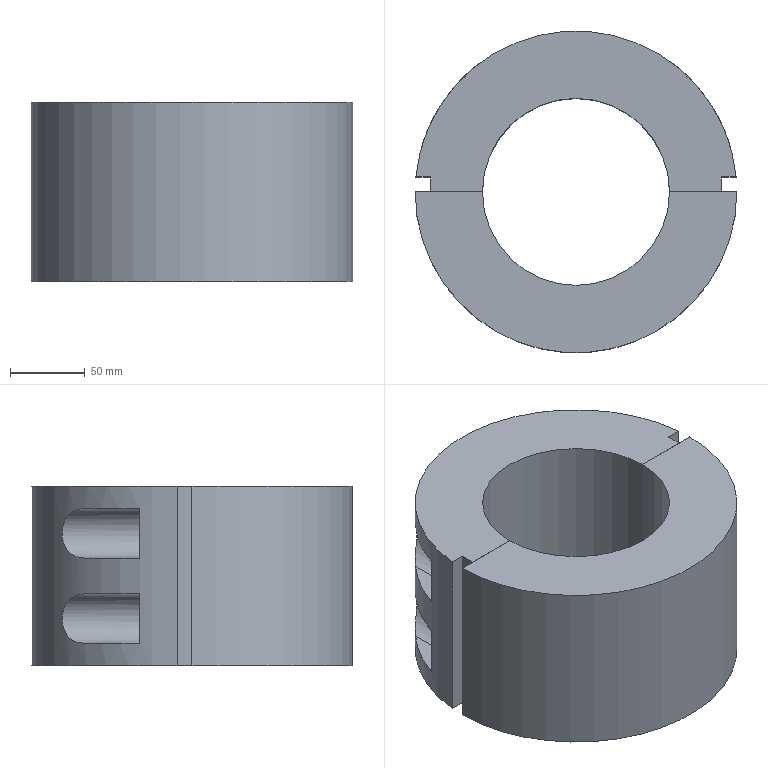NC program | NX | posted with a generic post | part box 215 x 215 x 120 mm
Lines 1 to 978 of 5839:
N10 G17 G21 G94 G90
(ZLEVEL_PROFILE , TOOL : D25)
N12 T01 M6
N14 G54
N16 G17 G0 G90 X-84.857 Y27.341 S1000 M3
N18 G43 Z30. H1
N20 Z-20.759
N22 G94 G1 X-80.33 Y25.016 F2000.
N24 G3 X-77.833 Y25.138 R2.5
N26 X-77.839 Y31.866 R4.
N28 X-80.336 Y31.984 R2.5
N30 G1 X-84.852 Y29.654
N32 G0 X-84.889 Y27.512 Z-21.109
N34 G1 X-80.453 Y25.029
N36 G3 X-77.954 Y25.063 R2.5
N38 X-77.949 Y31.934 R4.
N40 X-80.449 Y31.971 R2.5
N42 G1 X-84.894 Y29.491
N44 G0 X-84.922 Y27.671 Z-21.458
N46 G1 X-80.565 Y25.046
N48 G3 X-78.065 Y24.999 R2.5
N50 X-78.061 Y31.999 R4.
N52 X-80.561 Y31.955 R2.5
N54 G1 X-84.925 Y29.331
N56 G0 X-84.953 Y27.824 Z-21.808
N58 G1 X-80.668 Y25.064
N60 G3 X-78.171 Y24.943 R2.5
N62 X-78.173 Y32.058 R4.
N64 X-80.67 Y31.935 R2.5
N66 G1 X-84.947 Y29.176
N68 G0 X-84.96 Y27.979 Z-22.158
N70 G1 X-80.781 Y25.088
N72 G3 X-78.289 Y24.884 R2.5
N74 X-78.28 Y32.111 R4.
N76 X-80.773 Y31.914 R2.5
N78 G1 X-84.968 Y29.026
N80 G0 X-84.979 Y28.124 Z-22.507
N82 G1 X-80.876 Y25.111
N84 G3 X-78.391 Y24.838 R2.5
N86 X-78.397 Y32.165 R4.
N88 X-80.882 Y31.887 R2.5
N90 G1 X-84.975 Y28.872
N92 G0 X-84.991 Y28.266 Z-22.857
N94 G1 X-80.97 Y25.137
N96 G3 X-78.494 Y24.794 R2.5
N98 X-78.504 Y32.21 R4.
N100 X-80.979 Y31.86 R2.5
N102 G1 X-84.983 Y28.728
N104 G0 X-84.993 Y28.408 Z-23.206
N106 G1 X-81.068 Y25.167
N108 G3 X-78.603 Y24.752 R2.5
N110 X-78.601 Y32.247 R4.
N112 X-81.067 Y31.834 R2.5
N114 G1 X-84.994 Y28.592
N116 G0 X-89.054 Y32.079 Z-23.556
N118 G1 X-81.156 Y25.196
N120 G3 X-78.702 Y24.716 R2.5
N122 X-78.7 Y32.283 R4.
N124 X-81.154 Y31.804 R2.5
N126 G1 X-89.065 Y24.919
N128 G0 X-85.266 Y28.501 Z-23.906
N130 G1 X-81.25 Y25.231
N132 G3 X-78.811 Y24.681 R2.5
N134 X-78.811 Y32.319 R4.
N136 X-81.25 Y31.769 R2.5
N138 G1 X-85.266 Y28.501
N140 G0 X-85.496 Z-24.255
N142 G1 X-81.34 Y25.267
N144 G3 X-78.917 Y24.649 R2.5
N146 X-78.909 Y32.348 R4.
N148 X-81.333 Y31.736 R2.5
N150 G1 X-85.496 Y28.501
N152 G0 X-85.732 Y28.5 Z-24.605
N154 G1 X-81.42 Y25.301
N156 G3 X-79.014 Y24.623 R2.5
N158 X-79.008 Y32.375 R4.
N160 X-81.416 Y31.701 R2.5
N162 G1 X-85.732 Y28.5
N164 G0 X-85.978 Z-24.954
N166 G1 X-81.499 Y25.337
N168 G3 X-79.111 Y24.6 R2.5
N170 X-79.108 Y32.399 R4.
N172 X-81.497 Y31.664 R2.5
N174 G1 X-85.978 Y28.5
N176 G0 X-86.23 Z-25.304
N178 G1 X-81.574 Y25.374
N180 G3 X-79.203 Y24.58 R2.5
N182 X-79.208 Y32.421 R4.
N184 X-81.578 Y31.624 R2.5
N186 G1 X-86.23 Y28.5
N188 G0 X-86.491 Z-25.654
N190 G1 X-81.653 Y25.415
N192 G3 X-79.303 Y24.561 R2.5
N194 X-79.303 Y32.439 R4.
N196 X-81.653 Y31.585 R2.5
N198 G1 X-86.491 Y28.5
N200 G0 X-86.763 Z-26.003
N202 G1 X-81.714 Y25.448
N204 G3 X-79.381 Y24.548 R2.5
N206 X-79.385 Y32.452 R4.
N208 X-81.716 Y31.55 R2.5
N210 G1 X-86.763 Y28.5
N212 G0 X-87.061 Y28.501 Z-26.353
N214 G1 X-81.799 Y25.498
N216 G3 X-79.493 Y24.532 R2.5
N218 X-79.492 Y32.468 R4.
N220 X-81.798 Y31.503 R2.5
N222 G1 X-87.061 Y28.501
N224 G0 X-87.378 Y28.499 Z-26.702
N226 G1 X-81.868 Y25.54
N228 G3 X-79.585 Y24.522 R2.5
N230 X-79.67 Y32.486 R4.
N232 X-81.931 Y31.419 R2.5
N234 G1 X-87.378 Y28.499
N236 G0 X-87.666 Y28.5 Z-27.052
N238 G1 X-81.925 Y25.577
N240 G3 X-79.662 Y24.514 R2.5
N242 X-79.67 Y32.486 R4.
N244 X-81.931 Y31.419 R2.5
N246 G1 X-87.666 Y28.5
N248 G0 X-87.966 Z-27.402
N250 G1 X-81.991 Y25.621
N252 G3 X-79.752 Y24.508 R2.5
N254 X-79.769 Y32.493 R4.
N256 X-82.003 Y31.37 R2.5
N258 G1 X-87.966 Y28.5
N260 G0 X-88.287 Y28.501 Z-27.751
N262 G1 X-82.048 Y25.662
N264 G3 X-79.833 Y24.503 R2.5
N266 X-79.835 Y32.497 R4.
N268 X-82.05 Y31.337 R2.5
N270 G1 X-88.287 Y28.501
N272 G0 X-88.653 Z-28.101
N274 G1 X-82.114 Y25.71
N276 G3 X-79.926 Y24.501 R2.5
N278 X-79.927 Y32.499 R4.
N280 X-82.114 Y31.289 R2.5
N282 G1 X-88.653 Y28.501
N284 G0 X-89.027 Y28.5 Z-28.45
N286 G1 X-82.225 Y25.75
N288 G3 X-80.06 Y24.5 R2.5
N290 G1 X-80.
N292 G3 X-76. Y28.5 R4.
N294 X-80. Y32.5 R4.
N296 G1 X-80.112
N298 G3 X-82.277 Y31.25 R2.5
N300 G1 X-89.027 Y28.5
N302 G0 X-89.347 Y28.499 Z-28.8
N304 G1 X-82.598 Y25.75
N306 G3 X-80.433 Y24.5 R2.5
N308 G1 X-80.
N310 G3 X-76. Y28.5 R4.
N312 X-80. Y32.5 R4.
N314 G1 X-80.247
N316 G3 X-82.412 Y31.25 R2.5
N318 G1 X-89.347 Y28.499
N320 G0 X-89.666 Y28.5 Z-29.15
N322 G1 X-82.923 Y25.75
N324 G3 X-80.758 Y24.5 R2.5
N326 G1 X-80.
N328 G3 X-76. Y28.5 R4.
N330 X-80. Y32.5 R4.
N332 G1 X-80.654
N334 G3 X-82.819 Y31.25 R2.5
N336 G1 X-89.666 Y28.5
N338 G0 X-89.982 Y28.498 Z-29.499
N340 G1 X-83.238 Y25.75
N342 G3 X-81.073 Y24.5 R2.5
N344 G1 X-80.
N346 G3 X-76. Y28.5 R4.
N348 X-80. Y32.5 R4.
N350 G1 X-81.073
N352 G3 X-83.238 Y31.25 R2.5
N354 G1 X-89.982 Y28.498
N356 G0 X-90.302 Y28.502 Z-29.849
N358 G1 X-83.396 Y25.75
N360 G3 X-81.231 Y24.5 R2.5
N362 G1 X-80.
N364 G3 X-76. Y28.5 R4.
N366 X-80. Y32.5 R4.
N368 G1 X-81.24
N370 G3 X-83.405 Y31.25 R2.5
N372 G1 X-90.302 Y28.502
N374 G0 X-90.62 Y28.498 Z-30.198
N376 G1 X-83.848 Y25.75
N378 G3 X-81.683 Y24.5 R2.5
N380 G1 X-80.
N382 G3 X-76. Y28.5 R4.
N384 X-80. Y32.5 R4.
N386 G1 X-81.709
N388 G3 X-83.874 Y31.25 R2.5
N390 G1 X-90.62 Y28.498
N392 G0 X-90.942 Y28.5 Z-30.548
N394 G1 X-84.163 Y25.75
N396 G3 X-81.998 Y24.5 R2.5
N398 G1 X-80.
N400 G3 X-76. Y28.5 R4.
N402 X-80. Y32.5 R4.
N404 G1 X-82.022
N406 G3 X-84.187 Y31.25 R2.5
N408 G1 X-90.942 Y28.5
N410 G0 X-91.26 Y28.499 Z-30.898
N412 G1 X-84.514 Y25.75
N414 G3 X-82.349 Y24.5 R2.5
N416 G1 X-80.
N418 G3 X-76. Y28.5 R4.
N420 X-80. Y32.5 R4.
N422 G1 X-82.345
N424 G3 X-84.51 Y31.25 R2.5
N426 G1 X-91.26 Y28.499
N428 G0 X-91.581 Y28.5 Z-31.247
N430 G1 X-84.827 Y25.75
N432 G3 X-82.662 Y24.5 R2.5
N434 G1 X-80.
N436 G3 X-76. Y28.5 R4.
N438 X-80. Y32.5 R4.
N440 G1 X-82.666
N442 G3 X-84.831 Y31.25 R2.5
N444 G1 X-91.581 Y28.5
N446 G0 X-91.9 Z-31.597
N448 G1 X-84.986 Y25.75
N450 G3 X-82.821 Y24.5 R2.5
N452 G1 X-80.
N454 G3 X-76. Y28.5 R4.
N456 X-80. Y32.5 R4.
N458 G1 X-82.985
N460 G3 X-85.15 Y31.25 R2.5
N462 G1 X-91.9 Y28.5
N464 G0 X-92.217 Y28.498 Z-31.946
N466 G1 X-85.406 Y25.75
N468 G3 X-83.241 Y24.5 R2.5
N470 G1 X-80.
N472 G3 X-76. Y28.5 R4.
N474 X-80. Y32.5 R4.
N476 G1 X-83.259
N478 G3 X-85.424 Y31.25 R2.5
N480 G1 X-92.217 Y28.498
N482 G0 X-92.537 Y28.5 Z-32.296
N484 G1 X-85.725 Y25.75
N486 G3 X-83.56 Y24.5 R2.5
N488 G1 X-80.
N490 G3 X-76. Y28.5 R4.
N492 X-80. Y32.5 R4.
N494 G1 X-83.403
N496 G3 X-85.568 Y31.25 R2.5
N498 G1 X-92.537 Y28.5
N500 G0 X-92.858 Z-32.646
N502 G1 X-86.109 Y25.75
N504 G3 X-83.944 Y24.5 R2.5
N506 G1 X-80.
N508 G3 X-76. Y28.5 R4.
N510 X-80. Y32.5 R4.
N512 G1 X-83.928
N514 G3 X-86.094 Y31.25 R2.5
N516 G1 X-92.858 Y28.5
N518 G0 X-93.176 Z-32.995
N520 G1 X-86.435 Y25.75
N522 G3 X-84.27 Y24.5 R2.5
N524 G1 X-80.
N526 G3 X-76. Y28.5 R4.
N528 X-80. Y32.5 R4.
N530 G1 X-84.217
N532 G3 X-86.382 Y31.25 R2.5
N534 G1 X-93.176 Y28.5
N536 G0 X-93.493 Y28.499 Z-33.345
N538 G1 X-86.653 Y25.75
N540 G3 X-84.487 Y24.5 R2.5
N542 G1 X-80.
N544 G3 X-76. Y28.5 R4.
N546 X-80. Y32.5 R4.
N548 G1 X-84.536
N550 G3 X-86.701 Y31.25 R2.5
N552 G1 X-93.493 Y28.499
N554 G0 X-93.807 Y28.5 Z-33.694
N556 G1 X-86.976 Y25.75
N558 G3 X-84.811 Y24.5 R2.5
N560 G1 X-80.
N562 G3 X-76. Y28.5 R4.
N564 X-80. Y32.5 R4.
N566 G1 X-84.827
N568 G3 X-86.992 Y31.25 R2.5
N570 G1 X-93.807 Y28.5
N572 G0 X-94.102 Z-34.044
N574 G1 X-87.365 Y25.75
N576 G3 X-85.2 Y24.5 R2.5
N578 G1 X-80.
N580 G3 X-76. Y28.5 R4.
N582 X-80. Y32.5 R4.
N584 G1 X-85.196
N586 G3 X-87.361 Y31.25 R2.5
N588 G1 X-94.102 Y28.5
N590 G0 X-94.397 Y28.499 Z-34.394
N592 G1 X-87.387 Y25.75
N594 G3 X-85.222 Y24.5 R2.5
N596 G1 X-80.
N598 G3 X-76. Y28.5 R4.
N600 X-80. Y32.5 R4.
N602 G1 X-85.473
N604 G3 X-87.638 Y31.25 R2.5
N606 G1 X-94.397 Y28.499
N608 G0 X-94.698 Y28.5 Z-34.743
N610 G1 X-87.828 Y25.75
N612 G3 X-85.663 Y24.5 R2.5
N614 G1 X-80.
N616 G3 X-76. Y28.5 R4.
N618 X-80. Y32.5 R4.
N620 G1 X-85.782
N622 G3 X-87.947 Y31.25 R2.5
N624 G1 X-94.698 Y28.5
N626 G0 X-94.993 Y28.501 Z-35.093
N628 G1 X-88.235 Y25.75
N630 G3 X-86.07 Y24.5 R2.5
N632 G1 X-80.
N634 G3 X-76. Y28.5 R4.
N636 X-80. Y32.5 R4.
N638 G1 X-86.051
N640 G3 X-88.216 Y31.25 R2.5
N642 G1 X-94.993 Y28.501
N644 G0 X-95.288 Z-35.442
N646 G1 X-88.549 Y25.75
N648 G3 X-86.384 Y24.5 R2.5
N650 G1 X-80.
N652 G3 X-76. Y28.5 R4.
N654 X-80. Y32.5 R4.
N656 G1 X-86.341
N658 G3 X-88.506 Y31.25 R2.5
N660 G1 X-95.288 Y28.501
N662 G0 X-95.587 Y28.5 Z-35.792
N664 G1 X-88.779 Y25.75
N666 G3 X-86.614 Y24.5 R2.5
N668 G1 X-80.
N670 G3 X-76. Y28.5 R4.
N672 X-80. Y32.5 R4.
N674 G1 X-86.656
N676 G3 X-88.821 Y31.25 R2.5
N678 G1 X-95.587 Y28.5
N680 G0 X-95.872 Z-36.142
N682 G1 X-89.097 Y25.75
N684 G3 X-86.932 Y24.5 R2.5
N686 G1 X-80.
N688 G3 X-76. Y28.5 R4.
N690 X-80. Y32.5 R4.
N692 G1 X-86.944
N694 G3 X-89.109 Y31.25 R2.5
N696 G1 X-95.872 Y28.5
N698 G0 X-96.15 Y28.499 Z-36.491
N700 G1 X-89.412 Y25.75
N702 G3 X-87.247 Y24.5 R2.5
N704 G1 X-80.
N706 G3 X-76. Y28.5 R4.
N708 X-80. Y32.5 R4.
N710 G1 X-87.247
N712 G3 X-89.412 Y31.25 R2.5
N714 G1 X-96.15 Y28.499
N716 G0 X-96.434 Z-36.841
N718 G1 X-89.642 Y25.75
N720 G3 X-87.477 Y24.5 R2.5
N722 G1 X-80.
N724 G3 X-76. Y28.5 R4.
N726 X-80. Y32.5 R4.
N728 G1 X-87.433
N730 G3 X-89.599 Y31.25 R2.5
N732 G1 X-96.434 Y28.499
N734 G0 X-96.714 Z-37.19
N736 G1 X-89.958 Y25.75
N738 G3 X-87.793 Y24.5 R2.5
N740 G1 X-80.
N742 G3 X-76. Y28.5 R4.
N744 X-80. Y32.5 R4.
N746 G1 X-87.727
N748 G3 X-89.892 Y31.25 R2.5
N750 G1 X-96.714 Y28.499
N752 G0 X-96.993 Y28.5 Z-37.54
N754 G1 X-90.161 Y25.75
N756 G3 X-87.996 Y24.5 R2.5
N758 G1 X-80.
N760 G3 X-76. Y28.5 R4.
N762 X-80. Y32.5 R4.
N764 G1 X-87.976
N766 G3 X-90.141 Y31.25 R2.5
N768 G1 X-96.993 Y28.5
N770 G0 X-97.274 Z-37.89
N772 G1 X-90.508 Y25.75
N774 G3 X-88.342 Y24.5 R2.5
N776 G1 X-80.
N778 G3 X-76. Y28.5 R4.
N780 X-80. Y32.5 R4.
N782 G1 X-88.319
N784 G3 X-90.484 Y31.25 R2.5
N786 G1 X-97.274 Y28.5
N788 G0 X-97.554 Z-38.239
N790 G1 X-90.803 Y25.75
N792 G3 X-88.638 Y24.5 R2.5
N794 G1 X-80.
N796 G3 X-76. Y28.5 R4.
N798 X-80. Y32.5 R4.
N800 G1 X-88.646
N802 G3 X-90.811 Y31.25 R2.5
N804 G1 X-97.554 Y28.5
N806 G0 X-97.824 Z-38.589
N808 G1 X-91.002 Y25.75
N810 G3 X-88.837 Y24.5 R2.5
N812 G1 X-80.
N814 G3 X-76. Y28.5 R4.
N816 X-80. Y32.5 R4.
N818 G1 X-88.859
N820 G3 X-91.024 Y31.25 R2.5
N822 G1 X-97.824 Y28.5
N824 G0 X-98.085 Y28.501 Z-38.938
N826 G1 X-91.166 Y25.75
N828 G3 X-89.001 Y24.5 R2.5
N830 G1 X-80.
N832 G3 X-76. Y28.5 R4.
N834 X-80. Y32.5 R4.
N836 G1 X-89.168
N838 G3 X-91.333 Y31.25 R2.5
N840 G1 X-98.085 Y28.501
N842 G0 X-98.354 Y28.5 Z-39.288
N844 G1 X-91.612 Y25.75
N846 G3 X-89.447 Y24.5 R2.5
N848 G1 X-80.
N850 G3 X-76. Y28.5 R4.
N852 X-80. Y32.5 R4.
N854 G1 X-89.445
N856 G3 X-91.61 Y31.25 R2.5
N858 G1 X-98.354 Y28.5
N860 G0 X-98.619 Y28.499 Z-39.638
N862 G1 X-91.797 Y25.75
N864 G3 X-89.632 Y24.5 R2.5
N866 G1 X-80.
N868 G3 X-76. Y28.5 R4.
N870 X-80. Y32.5 R4.
N872 G1 X-89.645
N874 G3 X-91.81 Y31.25 R2.5
N876 G1 X-98.619 Y28.499
N878 G0 X-98.881 Y28.5 Z-39.987
N880 G1 X-92.117 Y25.75
N882 G3 X-89.952 Y24.5 R2.5
N884 G1 X-80.
N886 G3 X-76. Y28.5 R4.
N888 X-80. Y32.5 R4.
N890 G1 X-89.957
N892 G3 X-92.122 Y31.25 R2.5
N894 G1 X-98.881 Y28.5
N896 G0 X-99.148 Z-40.337
N898 G1 X-92.359 Y25.75
N900 G3 X-90.194 Y24.5 R2.5
N902 G1 X-80.
N904 G3 X-76. Y28.5 R4.
N906 X-80. Y32.5 R4.
N908 G1 X-90.23
N910 G3 X-92.395 Y31.25 R2.5
N912 G1 X-99.148 Y28.5
N914 G0 X-99.414 Z-40.686
N916 G1 X-92.585 Y25.75
N918 G3 X-90.42 Y24.5 R2.5
N920 G1 X-80.
N922 G3 X-76. Y28.5 R4.
N924 X-80. Y32.5 R4.
N926 G1 X-90.506
N928 G3 X-92.671 Y31.25 R2.5
N930 G1 X-99.414 Y28.5
N932 G0 X-99.669 Y28.501 Z-41.036
N934 G1 X-92.714 Y25.75
N936 G3 X-90.549 Y24.5 R2.5
N938 G1 X-80.
N940 G3 X-76. Y28.5 R4.
N942 X-80. Y32.5 R4.
N944 G1 X-90.756
N946 G3 X-92.921 Y31.25 R2.5
N948 G1 X-99.669 Y28.501
N950 G0 X-99.915 Z-41.386
N952 G1 X-93.155 Y25.75
N954 G3 X-90.99 Y24.5 R2.5
N956 G1 X-80.
N958 G3 X-76. Y28.5 R4.
N960 X-80. Y32.5 R4.
N962 G1 X-90.974
N964 G3 X-93.139 Y31.25 R2.5
N966 G1 X-99.915 Y28.501
N968 G0 X-100.168 Y28.5 Z-41.735
N970 G1 X-93.422 Y25.75
N972 G3 X-91.257 Y24.5 R2.5
N974 G1 X-80.
N976 G3 X-76. Y28.5 R4.
N978 X-80. Y32.5 R4.
N980 G1 X-91.181
N982 G3 X-93.346 Y31.25 R2.5
N984 G1 X-100.168 Y28.5
N986 G0 X-100.417 Y28.498 Z-42.085
N988 G1 X-93.674 Y25.75
N990 G3 X-91.509 Y24.5 R2.5
N992 G1 X-80.
N994 G3 X-76. Y28.5 R4.
N996 X-80. Y32.5 R4.
N998 G1 X-91.493
N1000 G3 X-93.658 Y31.25 R2.5
N1002 G1 X-100.417 Y28.498
N1004 G0 X-100.669 Y28.5 Z-42.434
N1006 G1 X-93.894 Y25.75
N1008 G3 X-91.729 Y24.5 R2.5
N1010 G1 X-80.
N1012 G3 X-76. Y28.5 R4.
N1014 X-80. Y32.5 R4.
N1016 G1 X-91.694
N1018 G3 X-93.859 Y31.25 R2.5
N1020 G1 X-100.669 Y28.5
N1022 G0 X-100.918 Z-42.784
N1024 G1 X-94.117 Y25.75
N1026 G3 X-91.952 Y24.5 R2.5
N1028 G1 X-80.
N1030 G3 X-76. Y28.5 R4.
N1032 X-80. Y32.5 R4.
N1034 G1 X-91.972
N1036 G3 X-94.137 Y31.25 R2.5
N1038 G1 X-100.918 Y28.5
N1040 G0 X-101.169 Z-43.134
N1042 G1 X-94.424 Y25.75
N1044 G3 X-92.259 Y24.5 R2.5
N1046 G1 X-80.
N1048 G3 X-76. Y28.5 R4.
N1050 X-80. Y32.5 R4.
N1052 G1 X-92.207
N1054 G3 X-94.372 Y31.25 R2.5
N1056 G1 X-101.169 Y28.5
N1058 G0 X-101.411 Z-43.483
N1060 G1 X-94.561 Y25.75
N1062 G3 X-92.396 Y24.5 R2.5
N1064 G1 X-80.
N1066 G3 X-76. Y28.5 R4.
N1068 X-80. Y32.5 R4.
N1070 G1 X-92.423
N1072 G3 X-94.588 Y31.25 R2.5
N1074 G1 X-101.411 Y28.5
N1076 G0 X-101.644 Y28.501 Z-43.833
N1078 G1 X-94.809 Y25.75
N1080 G3 X-92.644 Y24.5 R2.5
N1082 G1 X-80.
N1084 G3 X-76. Y28.5 R4.
N1086 X-80. Y32.5 R4.
N1088 G1 X-92.652
N1090 G3 X-94.817 Y31.25 R2.5
N1092 G1 X-101.644 Y28.501
N1094 G0 X-101.884 Y28.5 Z-44.182
N1096 G1 X-95.126 Y25.75
N1098 G3 X-92.961 Y24.5 R2.5
N1100 G1 X-80.
N1102 G3 X-76. Y28.5 R4.
N1104 X-80. Y32.5 R4.
N1106 G1 X-92.977
N1108 G3 X-95.142 Y31.25 R2.5
N1110 G1 X-101.884 Y28.5
N1112 G0 X-102.12 Y28.499 Z-44.532
N1114 G1 X-95.239 Y25.75
N1116 G3 X-93.074 Y24.5 R2.5
N1118 G1 X-80.
N1120 G3 X-76. Y28.5 R4.
N1122 X-80. Y32.5 R4.
N1124 G1 X-93.091
N1126 G3 X-95.256 Y31.25 R2.5
N1128 G1 X-102.12 Y28.499
N1130 G0 X-102.355 Y28.501 Z-44.882
N1132 G1 X-95.509 Y25.75
N1134 G3 X-93.344 Y24.5 R2.5
N1136 G1 X-80.
N1138 G3 X-76. Y28.5 R4.
N1140 X-80. Y32.5 R4.
N1142 G1 X-93.348
N1144 G3 X-95.514 Y31.25 R2.5
N1146 G1 X-102.355 Y28.501
N1148 G0 X-102.593 Z-45.231
N1150 G1 X-95.832 Y25.75
N1152 G3 X-93.667 Y24.5 R2.5
N1154 G1 X-80.
N1156 G3 X-76. Y28.5 R4.
N1158 X-80. Y32.5 R4.
N1160 G1 X-93.678
N1162 G3 X-95.843 Y31.25 R2.5
N1164 G1 X-102.593 Y28.501
N1166 G0 X-102.829 Y28.5 Z-45.581
N1168 G1 X-95.946 Y25.75
N1170 G3 X-93.781 Y24.5 R2.5
N1172 G1 X-80.
N1174 G3 X-76. Y28.5 R4.
N1176 X-80. Y32.5 R4.
N1178 G1 X-93.807
N1180 G3 X-95.972 Y31.25 R2.5
N1182 G1 X-102.829 Y28.5
N1184 G0 X-103.056 Y28.499 Z-45.93
N1186 G1 X-96.218 Y25.75
N1188 G3 X-94.053 Y24.5 R2.5
N1190 G1 X-80.
N1192 G3 X-76. Y28.5 R4.
N1194 X-80. Y32.5 R4.
N1196 G1 X-94.059
N1198 G3 X-96.224 Y31.25 R2.5
N1200 G1 X-103.056 Y28.499
N1202 G0 X-103.28 Y28.501 Z-46.28
N1204 G1 X-96.489 Y25.75
N1206 G3 X-94.323 Y24.5 R2.5
N1208 G1 X-80.
N1210 G3 X-76. Y28.5 R4.
N1212 X-80. Y32.5 R4.
N1214 G1 X-94.331
N1216 G3 X-96.496 Y31.25 R2.5
N1218 G1 X-103.28 Y28.501
N1220 G0 X-103.502 Z-46.63
N1222 G1 X-96.715 Y25.75
N1224 G3 X-94.55 Y24.5 R2.5
N1226 G1 X-80.
N1228 G3 X-76. Y28.5 R4.
N1230 X-80. Y32.5 R4.
N1232 G1 X-94.541
N1234 G3 X-96.706 Y31.25 R2.5
N1236 G1 X-103.502 Y28.501
N1238 G0 X-103.728 Y28.5 Z-46.979
N1240 G1 X-96.941 Y25.75
N1242 G3 X-94.775 Y24.5 R2.5
N1244 G1 X-80.
N1246 G3 X-76. Y28.5 R4.
N1248 X-80. Y32.5 R4.
N1250 G1 X-94.8
N1252 G3 X-96.965 Y31.25 R2.5
N1254 G1 X-103.728 Y28.5
N1256 G0 X-103.951 Z-47.329
N1258 G1 X-97.205 Y25.75
N1260 G3 X-95.039 Y24.5 R2.5
N1262 G1 X-80.
N1264 G3 X-76. Y28.5 R4.
N1266 X-80. Y32.5 R4.
N1268 G1 X-95.04
N1270 G3 X-97.205 Y31.25 R2.5
N1272 G1 X-103.951 Y28.5
N1274 G0 X-104.17 Y28.502 Z-47.678
N1276 G1 X-97.425 Y25.75
N1278 G3 X-95.26 Y24.5 R2.5
N1280 G1 X-80.
N1282 G3 X-76. Y28.5 R4.
N1284 X-80. Y32.5 R4.
N1286 G1 X-95.155
N1288 G3 X-97.32 Y31.25 R2.5
N1290 G1 X-104.17 Y28.502
N1292 G0 X-104.396 Y28.5 Z-48.028
N1294 G1 X-97.651 Y25.75
N1296 G3 X-95.486 Y24.5 R2.5
N1298 G1 X-80.
N1300 G3 X-76. Y28.5 R4.
N1302 X-80. Y32.5 R4.
N1304 G1 X-95.404
N1306 G3 X-97.57 Y31.25 R2.5
N1308 G1 X-104.396 Y28.5
N1310 G0 X-104.615 Z-48.378
N1312 G1 X-97.87 Y25.75
N1314 G3 X-95.705 Y24.5 R2.5
N1316 G1 X-80.
N1318 G3 X-76. Y28.5 R4.
N1320 X-80. Y32.5 R4.
N1322 G1 X-95.705
N1324 G3 X-97.87 Y31.25 R2.5
N1326 G1 X-104.615 Y28.5
N1328 G0 X-104.824 Y28.501 Z-48.727
N1330 G1 X-97.984 Y25.75
N1332 G3 X-95.819 Y24.5 R2.5
N1334 G1 X-80.
N1336 G3 X-76. Y28.5 R4.
N1338 X-80. Y32.5 R4.
N1340 G1 X-95.862
N1342 G3 X-98.027 Y31.25 R2.5
N1344 G1 X-104.824 Y28.501
N1346 G0 X-105.033 Z-49.077
N1348 G1 X-98.228 Y25.75
N1350 G3 X-96.063 Y24.5 R2.5
N1352 G1 X-80.
N1354 G3 X-76. Y28.5 R4.
N1356 X-80. Y32.5 R4.
N1358 G1 X-96.079
N1360 G3 X-98.244 Y31.25 R2.5
N1362 G1 X-105.033 Y28.501
N1364 G0 X-105.245 Y28.5 Z-49.426
N1366 G1 X-98.458 Y25.75
N1368 G3 X-96.293 Y24.5 R2.5
N1370 G1 X-80.
N1372 G3 X-76. Y28.5 R4.
N1374 X-80. Y32.5 R4.
N1376 G1 X-96.292
N1378 G3 X-98.457 Y31.25 R2.5
N1380 G1 X-105.245 Y28.5
N1382 G0 X-105.455 Y28.499 Z-49.776
N1384 G1 X-98.62 Y25.75
N1386 G3 X-96.455 Y24.5 R2.5
N1388 G1 X-80.
N1390 G3 X-76. Y28.5 R4.
N1392 X-80. Y32.5 R4.
N1394 G1 X-96.548
N1396 G3 X-98.713 Y31.25 R2.5
N1398 G1 X-105.455 Y28.499
N1400 G0 X-105.662 Y28.502 Z-50.126
N1402 G1 X-98.917 Y25.75
N1404 G3 X-96.752 Y24.5 R2.5
N1406 G1 X-80.
N1408 G3 X-76. Y28.5 R4.
N1410 X-80. Y32.5 R4.
N1412 G1 X-96.58
N1414 G3 X-98.745 Y31.25 R2.5
N1416 G1 X-105.662 Y28.502
N1418 G0 X-105.873 Y28.5 Z-50.475
N1420 G1 X-99.039 Y25.75
N1422 G3 X-96.874 Y24.5 R2.5
N1424 G1 X-80.
N1426 G3 X-76. Y28.5 R4.
N1428 X-80. Y32.5 R4.
N1430 G1 X-96.883
N1432 G3 X-99.048 Y31.25 R2.5
N1434 G1 X-105.873 Y28.5
N1436 G0 X-106.083 Z-50.825
N1438 G1 X-99.337 Y25.75
N1440 G3 X-97.172 Y24.5 R2.5
N1442 G1 X-80.
N1444 G3 X-76. Y28.5 R4.
N1446 X-80. Y32.5 R4.
N1448 G1 X-97.128
N1450 G3 X-99.293 Y31.25 R2.5
N1452 G1 X-106.083 Y28.5
N1454 G0 X-106.285 Z-51.174
N1456 G1 X-99.528 Y25.75
N1458 G3 X-97.363 Y24.5 R2.5
N1460 G1 X-80.
N1462 G3 X-76. Y28.5 R4.
N1464 X-80. Y32.5 R4.
N1466 G1 X-97.341
N1468 G3 X-99.506 Y31.25 R2.5
N1470 G1 X-106.285 Y28.5
N1472 G0 X-106.482 Z-51.524
N1474 G1 X-99.735 Y25.75
N1476 G3 X-97.57 Y24.5 R2.5
N1478 G1 X-80.
N1480 G3 X-76. Y28.5 R4.
N1482 X-80. Y32.5 R4.
N1484 G1 X-97.572
N1486 G3 X-99.737 Y31.25 R2.5
N1488 G1 X-106.482 Y28.5
N1490 G0 X-106.679 Y28.499 Z-51.874
N1492 G1 X-99.86 Y25.75
N1494 G3 X-97.695 Y24.5 R2.5
N1496 G1 X-80.
N1498 G3 X-76. Y28.5 R4.
N1500 X-80. Y32.5 R4.
N1502 G1 X-97.677
N1504 G3 X-99.842 Y31.25 R2.5
N1506 G1 X-106.679 Y28.499
N1508 G0 X-106.878 Y28.5 Z-52.223
N1510 G1 X-100.029 Y25.75
N1512 G3 X-97.864 Y24.5 R2.5
N1514 G1 X-80.
N1516 G3 X-76. Y28.5 R4.
N1518 X-80. Y32.5 R4.
N1520 G1 X-97.965
N1522 G3 X-100.13 Y31.25 R2.5
N1524 G1 X-106.878 Y28.5
N1526 G0 X-107.074 Z-52.573
N1528 G1 X-100.166 Y25.75
N1530 G3 X-98.001 Y24.5 R2.5
N1532 G1 X-80.
N1534 G3 X-76. Y28.5 R4.
N1536 X-80. Y32.5 R4.
N1538 G1 X-98.07
N1540 G3 X-100.236 Y31.25 R2.5
N1542 G1 X-107.074 Y28.5
N1544 G0 X-107.267 Y28.501 Z-52.922
N1546 G1 X-100.458 Y25.75
N1548 G3 X-98.293 Y24.5 R2.5
N1550 G1 X-80.
N1552 G3 X-76. Y28.5 R4.
N1554 X-80. Y32.5 R4.
N1556 G1 X-98.31
N1558 G3 X-100.475 Y31.25 R2.5
N1560 G1 X-107.267 Y28.501
N1562 G0 X-107.467 Y28.5 Z-53.272
N1564 G1 X-100.717 Y25.75
N1566 G3 X-98.552 Y24.5 R2.5
N1568 G1 X-80.
N1570 G3 X-76. Y28.5 R4.
N1572 X-80. Y32.5 R4.
N1574 G1 X-98.562
N1576 G3 X-100.728 Y31.25 R2.5
N1578 G1 X-107.467 Y28.5
N1580 G0 X-107.662 Z-53.622
N1582 G1 X-100.798 Y25.75
N1584 G3 X-98.633 Y24.5 R2.5
N1586 G1 X-80.
N1588 G3 X-76. Y28.5 R4.
N1590 X-80. Y32.5 R4.
N1592 G1 X-98.719
N1594 G3 X-100.884 Y31.25 R2.5
N1596 G1 X-107.662 Y28.5
N1598 G0 X-107.848 Z-53.971
N1600 G1 X-101.056 Y25.75
N1602 G3 X-98.891 Y24.5 R2.5
N1604 G1 X-80.
N1606 G3 X-76. Y28.5 R4.
N1608 X-80. Y32.5 R4.
N1610 G1 X-98.926
N1612 G3 X-101.091 Y31.25 R2.5
N1614 G1 X-107.848 Y28.5
N1616 G0 X-108.033 Z-54.321
N1618 G1 X-101.282 Y25.75
N1620 G3 X-99.117 Y24.5 R2.5
N1622 G1 X-80.
N1624 G3 X-76. Y28.5 R4.
N1626 X-80. Y32.5 R4.
N1628 G1 X-99.125
N1630 G3 X-101.29 Y31.25 R2.5
N1632 G1 X-108.033 Y28.5
N1634 G0 X-108.217 Z-54.67
N1636 G1 X-101.471 Y25.75
N1638 G3 X-99.306 Y24.5 R2.5
N1640 G1 X-80.
N1642 G3 X-76. Y28.5 R4.
N1644 X-80. Y32.5 R4.
N1646 G1 X-99.309
N1648 G3 X-101.475 Y31.25 R2.5
N1650 G1 X-108.217 Y28.5
N1652 G0 X-108.403 Z-55.02
N1654 G1 X-101.607 Y25.75
N1656 G3 X-99.442 Y24.5 R2.5
N1658 G1 X-80.
N1660 G3 X-76. Y28.5 R4.
N1662 X-80. Y32.5 R4.
N1664 G1 X-99.414
N1666 G3 X-101.579 Y31.25 R2.5
N1668 G1 X-108.403 Y28.5
N1670 G0 X-108.588 Z-55.37
N1672 G1 X-101.726 Y25.75
N1674 G3 X-99.56 Y24.5 R2.5
N1676 G1 X-80.
N1678 G3 X-76. Y28.5 R4.
N1680 X-80. Y32.5 R4.
N1682 G1 X-99.549
N1684 G3 X-101.714 Y31.25 R2.5
N1686 G1 X-108.588 Y28.5
N1688 G0 X-108.773 Z-55.719
N1690 G1 X-101.982 Y25.75
N1692 G3 X-99.817 Y24.5 R2.5
N1694 G1 X-80.
N1696 G3 X-76. Y28.5 R4.
N1698 X-80. Y32.5 R4.
N1700 G1 X-99.814
N1702 G3 X-101.979 Y31.25 R2.5
N1704 G1 X-108.773 Y28.5
N1706 G0 X-108.956 Z-56.069
N1708 G1 X-102.202 Y25.75
N1710 G3 X-100.037 Y24.5 R2.5
N1712 G1 X-80.
N1714 G3 X-76. Y28.5 R4.
N1716 X-80. Y32.5 R4.
N1718 G1 X-100.039
N1720 G3 X-102.204 Y31.25 R2.5
N1722 G1 X-108.956 Y28.5
N1724 G0 X-109.137 Y28.499 Z-56.418
N1726 G1 X-102.349 Y25.75
N1728 G3 X-100.184 Y24.5 R2.5
N1730 G1 X-80.
N1732 G3 X-76. Y28.5 R4.
N1734 X-80. Y32.5 R4.
N1736 G1 X-100.218
N1738 G3 X-102.383 Y31.25 R2.5
N1740 G1 X-109.137 Y28.499
N1742 G0 X-109.31 Y28.5 Z-56.768
N1744 G1 X-102.56 Y25.75
N1746 G3 X-100.395 Y24.5 R2.5
N1748 G1 X-80.
N1750 G3 X-76. Y28.5 R4.
N1752 X-80. Y32.5 R4.
N1754 G1 X-100.397
N1756 G3 X-102.562 Y31.25 R2.5
N1758 G1 X-109.31 Y28.5
N1760 G0 X-109.481 Y28.499 Z-57.118
N1762 G1 X-102.685 Y25.75
N1764 G3 X-100.52 Y24.5 R2.5
N1766 G1 X-80.
N1768 G3 X-76. Y28.5 R4.
N1770 X-80. Y32.5 R4.
N1772 G1 X-100.515
N1774 G3 X-102.68 Y31.25 R2.5
N1776 G1 X-109.481 Y28.499
N1778 G0 X-109.655 Y28.5 Z-57.467
N1780 G1 X-102.89 Y25.75
N1782 G3 X-100.725 Y24.5 R2.5
N1784 G1 X-80.
N1786 G3 X-76. Y28.5 R4.
N1788 X-80. Y32.5 R4.
N1790 G1 X-100.7
N1792 G3 X-102.865 Y31.25 R2.5
N1794 G1 X-109.655 Y28.5
N1796 G0 X-109.828 Z-57.817
N1798 G1 X-103.004 Y25.75
N1800 G3 X-100.839 Y24.5 R2.5
N1802 G1 X-80.
N1804 G3 X-76. Y28.5 R4.
N1806 X-80. Y32.5 R4.
N1808 G1 X-100.819
N1810 G3 X-102.985 Y31.25 R2.5
N1812 G1 X-109.828 Y28.5
N1814 G0 X-110.001 Y28.499 Z-58.166
N1816 G1 X-103.131 Y25.75
N1818 G3 X-100.966 Y24.5 R2.5
N1820 G1 X-80.
N1822 G3 X-76. Y28.5 R4.
N1824 X-80. Y32.5 R4.
N1826 G1 X-100.967
N1828 G3 X-103.132 Y31.25 R2.5
N1830 G1 X-110.001 Y28.499
N1832 G0 X-110.178 Y28.502 Z-58.516
N1834 G1 X-103.393 Y25.75
N1836 G3 X-101.228 Y24.5 R2.5
N1838 G1 X-80.
N1840 G3 X-76. Y28.5 R4.
N1842 X-80. Y32.5 R4.
N1844 G1 X-101.229
N1846 G3 X-103.394 Y31.25 R2.5
N1848 G1 X-110.178 Y28.502
N1850 G0 X-110.345 Y28.5 Z-58.866
N1852 G1 X-103.958 Y25.666
N1854 G3 X-101.75 Y24.494 R2.5
N1856 G1 X-101.636 Y24.498
N1858 X-101.405 Y24.5
N1860 X-80.
N1862 G3 X-76. Y28.5 R4.
N1864 X-80. Y32.5 R4.
N1866 G1 X-101.407
N1868 X-101.647 Y32.503
N1870 X-101.729 Y32.505
N1872 G3 X-103.926 Y31.312 R2.5
N1874 G1 X-110.345 Y28.5
N1876 G0 X-110.509 Z-59.215
N1878 G1 X-104.105 Y25.697
N1880 G3 X-101.915 Y24.493 R2.5
N1882 G1 X-101.609 Y24.5
N1884 X-80.
N1886 G3 X-76. Y28.5 R4.
N1888 X-80. Y32.5 R4.
N1890 G1 X-101.609
N1892 X-101.642
N1894 X-101.647 Y32.502
N1896 X-101.893 Y32.508
N1898 G3 X-104.088 Y31.311 R2.5
N1900 G1 X-110.509 Y28.5
N1902 G0 X-110.673 Y28.499 Z-59.565
N1904 G1 X-104.305 Y25.634
N1906 G3 X-102.079 Y24.495 R2.5
N1908 G1 X-102.049 Y24.496
N1910 X-101.697
N1912 X-101.631 Y24.5
N1914 X-80.
N1916 G3 X-76. Y28.5 R4.
N1918 X-80. Y32.5 R4.
N1920 G1 X-101.642
N1922 X-101.653 Y32.503
N1924 X-102.058 Y32.504
N1926 G3 X-104.225 Y31.257 R2.5
N1928 G1 X-110.673 Y28.499
N1930 G0 X-110.832 Y28.501 Z-59.914
N1932 G1 X-104.426 Y25.704
N1934 G3 X-102.24 Y24.49 R2.5
N1936 G1 X-101.631 Y24.5
N1938 X-80.
N1940 G3 X-76. Y28.5 R4.
N1942 X-80. Y32.5 R4.
N1944 G1 X-101.642
N1946 X-102.219 Y32.51
N1948 G3 X-104.405 Y31.297 R2.5
N1950 G1 X-110.832 Y28.501
N1952 G0 X-110.998 Y28.499 Z-60.264
N1954 G1 X-104.585 Y25.706